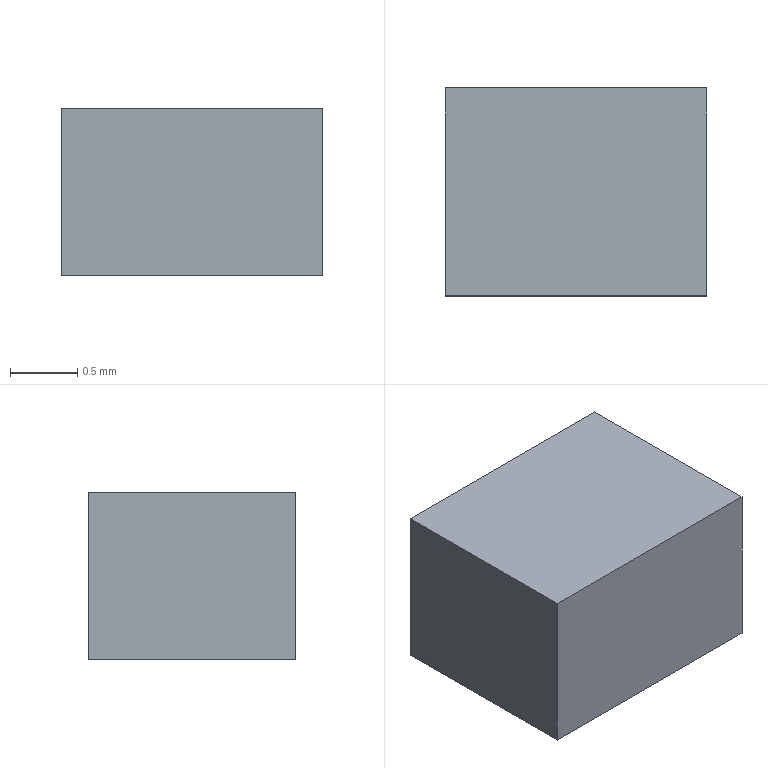Part | Creo | 1 solid | 6 faces | box 1.95 x 1.55 x 1.245 mm | volume 3.764 mm3 | plane 6
STEP:
#1=CARTESIAN_POINT('',(0.,0.,0.));
#2=DIRECTION('',(0.,0.,1.));
#3=DIRECTION('',(1.,0.,0.));
#4=AXIS2_PLACEMENT_3D('',#1,#2,#3);
#5=CARTESIAN_POINT('',(-1.025,-0.825,0.));
#6=VERTEX_POINT('',#5);
#7=CARTESIAN_POINT('',(0.925,-0.825,0.));
#8=VERTEX_POINT('',#7);
#9=CARTESIAN_POINT('',(-1.025,-0.825,0.));
#10=DIRECTION('',(1.,0.,0.));
#11=VECTOR('',#10,1.95);
#12=LINE('',#9,#11);
#13=EDGE_CURVE('',#6,#8,#12,.T.);
#14=ORIENTED_EDGE('',*,*,#13,.T.);
#15=CARTESIAN_POINT('',(0.925,0.725,0.));
#16=VERTEX_POINT('',#15);
#17=CARTESIAN_POINT('',(0.925,-0.825,0.));
#18=DIRECTION('',(0.,1.,0.));
#19=VECTOR('',#18,1.55);
#20=LINE('',#17,#19);
#21=EDGE_CURVE('',#8,#16,#20,.T.);
#22=ORIENTED_EDGE('',*,*,#21,.T.);
#23=CARTESIAN_POINT('',(-1.025,0.725,0.));
#24=VERTEX_POINT('',#23);
#25=CARTESIAN_POINT('',(0.925,0.725,0.));
#26=DIRECTION('',(-1.,0.,0.));
#27=VECTOR('',#26,1.95);
#28=LINE('',#25,#27);
#29=EDGE_CURVE('',#16,#24,#28,.T.);
#30=ORIENTED_EDGE('',*,*,#29,.T.);
#31=CARTESIAN_POINT('',(-1.025,0.725,0.));
#32=DIRECTION('',(0.,-1.,0.));
#33=VECTOR('',#32,1.55);
#34=LINE('',#31,#33);
#35=EDGE_CURVE('',#24,#6,#34,.T.);
#36=ORIENTED_EDGE('',*,*,#35,.T.);
#37=EDGE_LOOP('',(#14,#22,#30,#36));
#38=FACE_OUTER_BOUND('',#37,.F.);
#39=CARTESIAN_POINT('',(0.,0.,0.));
#40=DIRECTION('',(0.,0.,1.));
#41=DIRECTION('',(1.,0.,0.));
#42=AXIS2_PLACEMENT_3D('',#39,#40,#41);
#43=PLANE('',#42);
#44=ADVANCED_FACE('',(#38),#43,.F.);
#45=ORIENTED_EDGE('',*,*,#13,.F.);
#46=CARTESIAN_POINT('',(-1.025,-0.825,1.245));
#47=VERTEX_POINT('',#46);
#48=CARTESIAN_POINT('',(-1.025,-0.825,0.));
#49=DIRECTION('',(0.,0.,1.));
#50=VECTOR('',#49,1.245);
#51=LINE('',#48,#50);
#52=EDGE_CURVE('',#6,#47,#51,.T.);
#53=ORIENTED_EDGE('',*,*,#52,.T.);
#54=CARTESIAN_POINT('',(0.925,-0.825,1.245));
#55=VERTEX_POINT('',#54);
#56=CARTESIAN_POINT('',(-1.025,-0.825,1.245));
#57=DIRECTION('',(1.,0.,0.));
#58=VECTOR('',#57,1.95);
#59=LINE('',#56,#58);
#60=EDGE_CURVE('',#47,#55,#59,.T.);
#61=ORIENTED_EDGE('',*,*,#60,.T.);
#62=CARTESIAN_POINT('',(0.925,-0.825,0.));
#63=DIRECTION('',(0.,0.,1.));
#64=VECTOR('',#63,1.245);
#65=LINE('',#62,#64);
#66=EDGE_CURVE('',#8,#55,#65,.T.);
#67=ORIENTED_EDGE('',*,*,#66,.F.);
#68=EDGE_LOOP('',(#45,#53,#61,#67));
#69=FACE_OUTER_BOUND('',#68,.F.);
#70=CARTESIAN_POINT('',(-1.025,-0.825,0.));
#71=DIRECTION('',(0.,-1.,0.));
#72=DIRECTION('',(1.,0.,0.));
#73=AXIS2_PLACEMENT_3D('',#70,#71,#72);
#74=PLANE('',#73);
#75=ADVANCED_FACE('',(#69),#74,.T.);
#76=ORIENTED_EDGE('',*,*,#35,.F.);
#77=CARTESIAN_POINT('',(-1.025,0.725,1.245));
#78=VERTEX_POINT('',#77);
#79=CARTESIAN_POINT('',(-1.025,0.725,0.));
#80=DIRECTION('',(0.,0.,1.));
#81=VECTOR('',#80,1.245);
#82=LINE('',#79,#81);
#83=EDGE_CURVE('',#24,#78,#82,.T.);
#84=ORIENTED_EDGE('',*,*,#83,.T.);
#85=CARTESIAN_POINT('',(-1.025,0.725,1.245));
#86=DIRECTION('',(0.,-1.,0.));
#87=VECTOR('',#86,1.55);
#88=LINE('',#85,#87);
#89=EDGE_CURVE('',#78,#47,#88,.T.);
#90=ORIENTED_EDGE('',*,*,#89,.T.);
#91=ORIENTED_EDGE('',*,*,#52,.F.);
#92=EDGE_LOOP('',(#76,#84,#90,#91));
#93=FACE_OUTER_BOUND('',#92,.F.);
#94=CARTESIAN_POINT('',(-1.025,0.725,0.));
#95=DIRECTION('',(-1.,0.,0.));
#96=DIRECTION('',(0.,-1.,0.));
#97=AXIS2_PLACEMENT_3D('',#94,#95,#96);
#98=PLANE('',#97);
#99=ADVANCED_FACE('',(#93),#98,.T.);
#100=ORIENTED_EDGE('',*,*,#29,.F.);
#101=CARTESIAN_POINT('',(0.925,0.725,1.245));
#102=VERTEX_POINT('',#101);
#103=CARTESIAN_POINT('',(0.925,0.725,0.));
#104=DIRECTION('',(0.,0.,1.));
#105=VECTOR('',#104,1.245);
#106=LINE('',#103,#105);
#107=EDGE_CURVE('',#16,#102,#106,.T.);
#108=ORIENTED_EDGE('',*,*,#107,.T.);
#109=CARTESIAN_POINT('',(0.925,0.725,1.245));
#110=DIRECTION('',(-1.,0.,0.));
#111=VECTOR('',#110,1.95);
#112=LINE('',#109,#111);
#113=EDGE_CURVE('',#102,#78,#112,.T.);
#114=ORIENTED_EDGE('',*,*,#113,.T.);
#115=ORIENTED_EDGE('',*,*,#83,.F.);
#116=EDGE_LOOP('',(#100,#108,#114,#115));
#117=FACE_OUTER_BOUND('',#116,.F.);
#118=CARTESIAN_POINT('',(0.925,0.725,0.));
#119=DIRECTION('',(0.,1.,0.));
#120=DIRECTION('',(-1.,0.,0.));
#121=AXIS2_PLACEMENT_3D('',#118,#119,#120);
#122=PLANE('',#121);
#123=ADVANCED_FACE('',(#117),#122,.T.);
#124=ORIENTED_EDGE('',*,*,#21,.F.);
#125=ORIENTED_EDGE('',*,*,#66,.T.);
#126=CARTESIAN_POINT('',(0.925,-0.825,1.245));
#127=DIRECTION('',(0.,1.,0.));
#128=VECTOR('',#127,1.55);
#129=LINE('',#126,#128);
#130=EDGE_CURVE('',#55,#102,#129,.T.);
#131=ORIENTED_EDGE('',*,*,#130,.T.);
#132=ORIENTED_EDGE('',*,*,#107,.F.);
#133=EDGE_LOOP('',(#124,#125,#131,#132));
#134=FACE_OUTER_BOUND('',#133,.F.);
#135=CARTESIAN_POINT('',(0.925,-0.825,0.));
#136=DIRECTION('',(1.,0.,0.));
#137=DIRECTION('',(0.,1.,0.));
#138=AXIS2_PLACEMENT_3D('',#135,#136,#137);
#139=PLANE('',#138);
#140=ADVANCED_FACE('',(#134),#139,.T.);
#141=ORIENTED_EDGE('',*,*,#60,.F.);
#142=ORIENTED_EDGE('',*,*,#89,.F.);
#143=ORIENTED_EDGE('',*,*,#113,.F.);
#144=ORIENTED_EDGE('',*,*,#130,.F.);
#145=EDGE_LOOP('',(#141,#142,#143,#144));
#146=FACE_OUTER_BOUND('',#145,.F.);
#147=CARTESIAN_POINT('',(0.,0.,1.245));
#148=DIRECTION('',(0.,0.,1.));
#149=DIRECTION('',(1.,0.,0.));
#150=AXIS2_PLACEMENT_3D('',#147,#148,#149);
#151=PLANE('',#150);
#152=ADVANCED_FACE('',(#146),#151,.T.);
#153=CLOSED_SHELL('',(#44,#75,#99,#123,#140,#152));
#154=MANIFOLD_SOLID_BREP('',#153);
#155=(LENGTH_UNIT()NAMED_UNIT(*)SI_UNIT(.MILLI.,.METRE.));
#156=UNCERTAINTY_MEASURE_WITH_UNIT(LENGTH_MEASURE(0.0002785),#155,'','');
#157=(NAMED_UNIT(*)PLANE_ANGLE_UNIT()SI_UNIT($,.RADIAN.));
#158=PLANE_ANGLE_MEASURE_WITH_UNIT(PLANE_ANGLE_MEASURE(0.01745),#157);
#159=(CONVERSION_BASED_UNIT('DEGREE',#158)NAMED_UNIT(*)PLANE_ANGLE_UNIT());
#160=(NAMED_UNIT(*)SI_UNIT($,.STERADIAN.)SOLID_ANGLE_UNIT());
#161=(GEOMETRIC_REPRESENTATION_CONTEXT(3)GLOBAL_UNCERTAINTY_ASSIGNED_CONTEXT((#156))GLOBAL_UNIT_ASSIGNED_CONTEXT((#155,#159,#160))REPRESENTATION_CONTEXT('',''));
#162=ADVANCED_BREP_SHAPE_REPRESENTATION('',(#4,#154),#161);